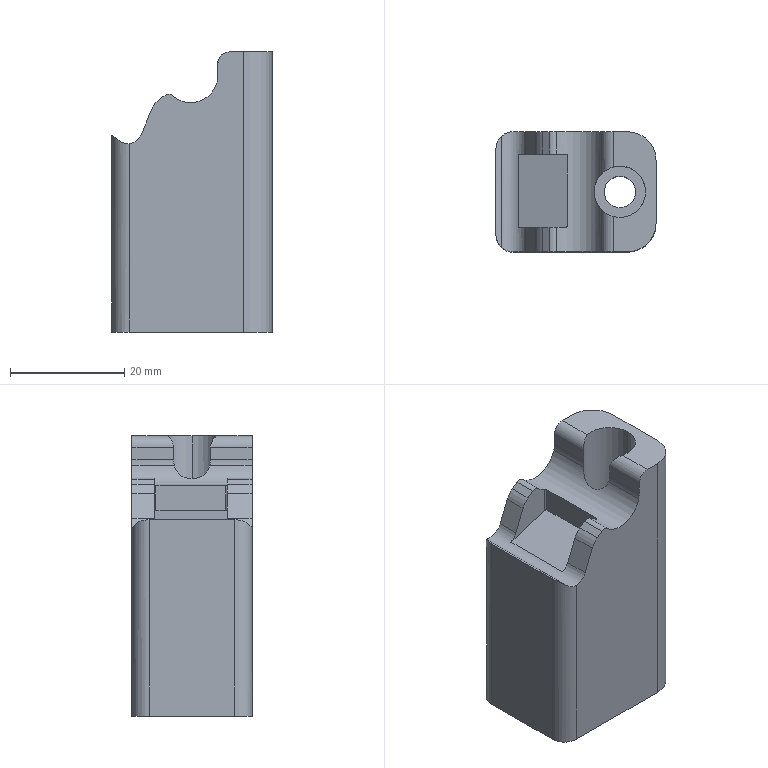Part | 1 solid | 38 faces | box 27.999 x 21 x 48.948 mm | volume 21596 mm3 | cylinder 20 | plane 17 | other 1 | commonest cylinder face diameters 9.5 x3 2 x2 4 x2 5.5 x2 6 x2 7.6 x2